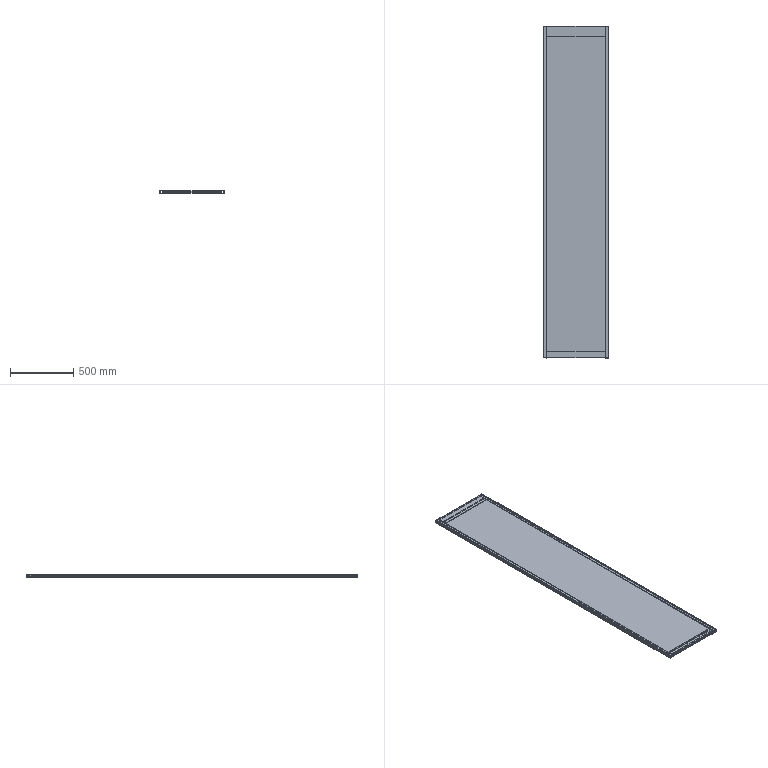Part | 5 solids | 330 faces | box 520 x 2616 x 20.2 mm | volume 13464411 mm3 | cylinder 180 | plane 150 | commonest cylinder face diameters 0.6 x48 13 x48 0.4 x27 1 x21 9 x16 7.2 x12